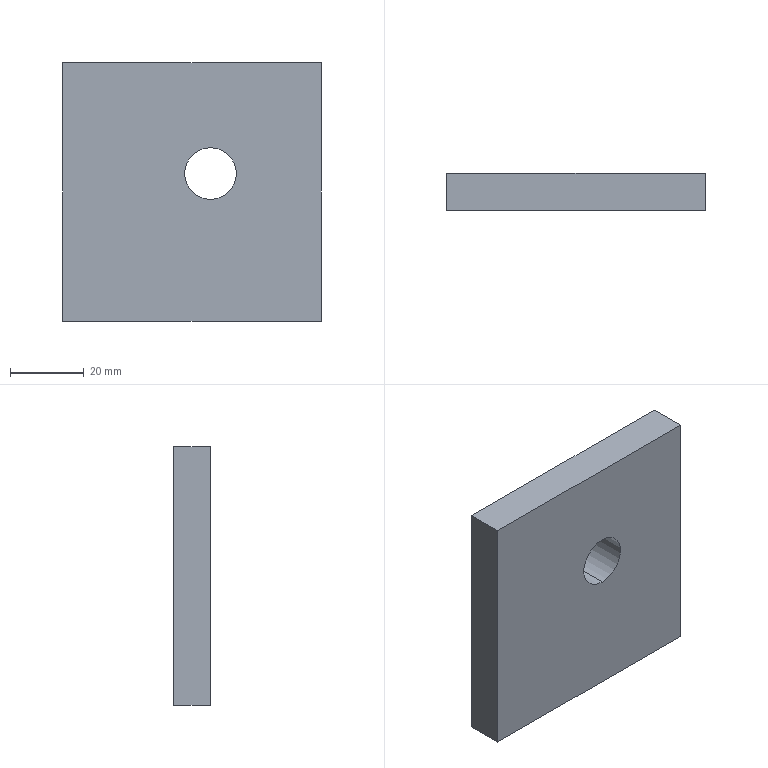Part | STEP file | PN_0078 foot-support plate | 1 solid | 8 faces | box 70 x 10 x 70 mm | volume 47461 mm3 | plane 6 | cylinder 2 | commonest cylinder face diameters 14 x2
STEP:
#1=CARTESIAN_POINT('',(0.,0.,0.));
#2=DIRECTION('',(0.,0.,1.));
#3=DIRECTION('',(1.,0.,0.));
#4=AXIS2_PLACEMENT_3D('',#1,#2,#3);
#5=CARTESIAN_POINT('',(-30.,0.,-23.));
#6=VERTEX_POINT('',#5);
#7=CARTESIAN_POINT('',(-30.,10.,-23.));
#8=VERTEX_POINT('',#7);
#9=CARTESIAN_POINT('',(-30.,10.,-23.));
#10=DIRECTION('',(0.,1.,0.));
#11=VECTOR('',#10,1.);
#12=LINE('',#9,#11);
#13=CARTESIAN_POINT('',(-30.,10.,-30.));
#14=DIRECTION('',(0.,1.,0.));
#15=DIRECTION('',(0.,0.,1.));
#16=AXIS2_PLACEMENT_3D('',#13,#14,#15);
#17=CYLINDRICAL_SURFACE('',#16,7.);
#18=CARTESIAN_POINT('',(6.283,0.));
#19=DIRECTION('',(0.,1.));
#20=VECTOR('',#19,1.);
#21=LINE('',#18,#20);
#22=(GEOMETRIC_REPRESENTATION_CONTEXT(2)PARAMETRIC_REPRESENTATION_CONTEXT()REPRESENTATION_CONTEXT('',''));
#23=DEFINITIONAL_REPRESENTATION('',(#21),#22);
#24=PCURVE('',#17,#23);
#25=CARTESIAN_POINT('',(-30.,10.,-30.));
#26=DIRECTION('',(0.,1.,0.));
#27=DIRECTION('',(0.,0.,1.));
#28=AXIS2_PLACEMENT_3D('',#25,#26,#27);
#29=CYLINDRICAL_SURFACE('',#28,7.);
#30=CARTESIAN_POINT('',(0.,0.));
#31=DIRECTION('',(0.,1.));
#32=VECTOR('',#31,1.);
#33=LINE('',#30,#32);
#34=(GEOMETRIC_REPRESENTATION_CONTEXT(2)PARAMETRIC_REPRESENTATION_CONTEXT()REPRESENTATION_CONTEXT('',''));
#35=DEFINITIONAL_REPRESENTATION('',(#33),#34);
#36=PCURVE('',#29,#35);
#37=SURFACE_CURVE('',#12,(#24,#36),.PCURVE_S1.);
#38=EDGE_CURVE('',#6,#8,#37,.T.);
#39=ORIENTED_EDGE('',*,*,#38,.T.);
#40=CARTESIAN_POINT('',(-30.,10.,-37.));
#41=VERTEX_POINT('',#40);
#42=CARTESIAN_POINT('',(-30.,10.,-30.));
#43=DIRECTION('',(0.,1.,0.));
#44=DIRECTION('',(0.,0.,1.));
#45=AXIS2_PLACEMENT_3D('',#42,#43,#44);
#46=CIRCLE('',#45,7.);
#47=CARTESIAN_POINT('',(0.,0.));
#48=DIRECTION('',(1.,0.));
#49=VECTOR('',#48,1.);
#50=LINE('',#47,#49);
#51=(GEOMETRIC_REPRESENTATION_CONTEXT(2)PARAMETRIC_REPRESENTATION_CONTEXT()REPRESENTATION_CONTEXT('',''));
#52=DEFINITIONAL_REPRESENTATION('',(#50),#51);
#53=PCURVE('',#17,#52);
#54=CARTESIAN_POINT('',(0.,10.,0.));
#55=DIRECTION('',(0.,1.,0.));
#56=DIRECTION('',(0.,0.,1.));
#57=AXIS2_PLACEMENT_3D('',#54,#55,#56);
#58=PLANE('',#57);
#59=CARTESIAN_POINT('',(-30.,-30.));
#60=DIRECTION('',(1.,0.));
#61=AXIS2_PLACEMENT_2D('',#59,#60);
#62=CIRCLE('',#61,7.);
#63=(GEOMETRIC_REPRESENTATION_CONTEXT(2)PARAMETRIC_REPRESENTATION_CONTEXT()REPRESENTATION_CONTEXT('',''));
#64=DEFINITIONAL_REPRESENTATION('',(#62),#63);
#65=PCURVE('',#58,#64);
#66=SURFACE_CURVE('',#46,(#53,#65),.PCURVE_S1.);
#67=EDGE_CURVE('',#41,#8,#66,.T.);
#68=ORIENTED_EDGE('',*,*,#67,.F.);
#69=CARTESIAN_POINT('',(-30.,0.,-37.));
#70=VERTEX_POINT('',#69);
#71=CARTESIAN_POINT('',(-30.,10.,-37.));
#72=DIRECTION('',(0.,1.,0.));
#73=VECTOR('',#72,1.);
#74=LINE('',#71,#73);
#75=CARTESIAN_POINT('',(3.142,0.));
#76=DIRECTION('',(0.,1.));
#77=VECTOR('',#76,1.);
#78=LINE('',#75,#77);
#79=(GEOMETRIC_REPRESENTATION_CONTEXT(2)PARAMETRIC_REPRESENTATION_CONTEXT()REPRESENTATION_CONTEXT('',''));
#80=DEFINITIONAL_REPRESENTATION('',(#78),#79);
#81=PCURVE('',#17,#80);
#82=CARTESIAN_POINT('',(3.142,0.));
#83=DIRECTION('',(0.,1.));
#84=VECTOR('',#83,1.);
#85=LINE('',#82,#84);
#86=(GEOMETRIC_REPRESENTATION_CONTEXT(2)PARAMETRIC_REPRESENTATION_CONTEXT()REPRESENTATION_CONTEXT('',''));
#87=DEFINITIONAL_REPRESENTATION('',(#85),#86);
#88=PCURVE('',#29,#87);
#89=SURFACE_CURVE('',#74,(#81,#88),.PCURVE_S1.);
#90=EDGE_CURVE('',#70,#41,#89,.T.);
#91=ORIENTED_EDGE('',*,*,#90,.F.);
#92=CARTESIAN_POINT('',(-30.,0.,-30.));
#93=DIRECTION('',(0.,1.,0.));
#94=DIRECTION('',(0.,0.,1.));
#95=AXIS2_PLACEMENT_3D('',#92,#93,#94);
#96=CIRCLE('',#95,7.);
#97=CARTESIAN_POINT('',(0.,-10.));
#98=DIRECTION('',(1.,0.));
#99=VECTOR('',#98,1.);
#100=LINE('',#97,#99);
#101=(GEOMETRIC_REPRESENTATION_CONTEXT(2)PARAMETRIC_REPRESENTATION_CONTEXT()REPRESENTATION_CONTEXT('',''));
#102=DEFINITIONAL_REPRESENTATION('',(#100),#101);
#103=PCURVE('',#17,#102);
#104=CARTESIAN_POINT('',(0.,0.,0.));
#105=DIRECTION('',(0.,1.,0.));
#106=DIRECTION('',(0.,0.,1.));
#107=AXIS2_PLACEMENT_3D('',#104,#105,#106);
#108=PLANE('',#107);
#109=CARTESIAN_POINT('',(-30.,-30.));
#110=DIRECTION('',(1.,0.));
#111=AXIS2_PLACEMENT_2D('',#109,#110);
#112=CIRCLE('',#111,7.);
#113=(GEOMETRIC_REPRESENTATION_CONTEXT(2)PARAMETRIC_REPRESENTATION_CONTEXT()REPRESENTATION_CONTEXT('',''));
#114=DEFINITIONAL_REPRESENTATION('',(#112),#113);
#115=PCURVE('',#108,#114);
#116=SURFACE_CURVE('',#96,(#103,#115),.PCURVE_S1.);
#117=EDGE_CURVE('',#70,#6,#116,.T.);
#118=ORIENTED_EDGE('',*,*,#117,.T.);
#119=EDGE_LOOP('',(#39,#68,#91,#118));
#120=FACE_BOUND('',#119,.F.);
#121=ADVANCED_FACE('',(#120),#17,.F.);
#122=CARTESIAN_POINT('',(0.,0.,0.));
#123=VERTEX_POINT('',#122);
#124=CARTESIAN_POINT('',(0.,0.,-70.));
#125=VERTEX_POINT('',#124);
#126=CARTESIAN_POINT('',(0.,0.,0.));
#127=DIRECTION('',(0.,0.,-1.));
#128=VECTOR('',#127,1.);
#129=LINE('',#126,#128);
#130=CARTESIAN_POINT('',(0.,10.,0.));
#131=DIRECTION('',(-1.,0.,0.));
#132=DIRECTION('',(0.,0.,1.));
#133=AXIS2_PLACEMENT_3D('',#130,#131,#132);
#134=PLANE('',#133);
#135=CARTESIAN_POINT('',(0.,-10.));
#136=DIRECTION('',(-1.,0.));
#137=VECTOR('',#136,1.);
#138=LINE('',#135,#137);
#139=(GEOMETRIC_REPRESENTATION_CONTEXT(2)PARAMETRIC_REPRESENTATION_CONTEXT()REPRESENTATION_CONTEXT('',''));
#140=DEFINITIONAL_REPRESENTATION('',(#138),#139);
#141=PCURVE('',#134,#140);
#142=CARTESIAN_POINT('',(0.,0.));
#143=DIRECTION('',(-1.,0.));
#144=VECTOR('',#143,1.);
#145=LINE('',#142,#144);
#146=(GEOMETRIC_REPRESENTATION_CONTEXT(2)PARAMETRIC_REPRESENTATION_CONTEXT()REPRESENTATION_CONTEXT('',''));
#147=DEFINITIONAL_REPRESENTATION('',(#145),#146);
#148=PCURVE('',#108,#147);
#149=SURFACE_CURVE('',#129,(#141,#148),.PCURVE_S1.);
#150=EDGE_CURVE('',#123,#125,#149,.T.);
#151=ORIENTED_EDGE('',*,*,#150,.T.);
#152=CARTESIAN_POINT('',(0.,10.,-70.));
#153=VERTEX_POINT('',#152);
#154=CARTESIAN_POINT('',(0.,10.,-70.));
#155=DIRECTION('',(0.,-1.,0.));
#156=VECTOR('',#155,1.);
#157=LINE('',#154,#156);
#158=CARTESIAN_POINT('',(-70.,0.));
#159=DIRECTION('',(0.,-1.));
#160=VECTOR('',#159,1.);
#161=LINE('',#158,#160);
#162=(GEOMETRIC_REPRESENTATION_CONTEXT(2)PARAMETRIC_REPRESENTATION_CONTEXT()REPRESENTATION_CONTEXT('',''));
#163=DEFINITIONAL_REPRESENTATION('',(#161),#162);
#164=PCURVE('',#134,#163);
#165=CARTESIAN_POINT('',(0.,10.,-70.));
#166=DIRECTION('',(0.,0.,1.));
#167=DIRECTION('',(1.,0.,0.));
#168=AXIS2_PLACEMENT_3D('',#165,#166,#167);
#169=PLANE('',#168);
#170=CARTESIAN_POINT('',(0.,0.));
#171=DIRECTION('',(0.,-1.));
#172=VECTOR('',#171,1.);
#173=LINE('',#170,#172);
#174=(GEOMETRIC_REPRESENTATION_CONTEXT(2)PARAMETRIC_REPRESENTATION_CONTEXT()REPRESENTATION_CONTEXT('',''));
#175=DEFINITIONAL_REPRESENTATION('',(#173),#174);
#176=PCURVE('',#169,#175);
#177=SURFACE_CURVE('',#157,(#164,#176),.PCURVE_S1.);
#178=EDGE_CURVE('',#153,#125,#177,.T.);
#179=ORIENTED_EDGE('',*,*,#178,.F.);
#180=CARTESIAN_POINT('',(0.,10.,0.));
#181=VERTEX_POINT('',#180);
#182=CARTESIAN_POINT('',(0.,10.,0.));
#183=DIRECTION('',(0.,0.,-1.));
#184=VECTOR('',#183,1.);
#185=LINE('',#182,#184);
#186=CARTESIAN_POINT('',(0.,0.));
#187=DIRECTION('',(-1.,0.));
#188=VECTOR('',#187,1.);
#189=LINE('',#186,#188);
#190=(GEOMETRIC_REPRESENTATION_CONTEXT(2)PARAMETRIC_REPRESENTATION_CONTEXT()REPRESENTATION_CONTEXT('',''));
#191=DEFINITIONAL_REPRESENTATION('',(#189),#190);
#192=PCURVE('',#134,#191);
#193=CARTESIAN_POINT('',(0.,0.));
#194=DIRECTION('',(-1.,0.));
#195=VECTOR('',#194,1.);
#196=LINE('',#193,#195);
#197=(GEOMETRIC_REPRESENTATION_CONTEXT(2)PARAMETRIC_REPRESENTATION_CONTEXT()REPRESENTATION_CONTEXT('',''));
#198=DEFINITIONAL_REPRESENTATION('',(#196),#197);
#199=PCURVE('',#58,#198);
#200=SURFACE_CURVE('',#185,(#192,#199),.PCURVE_S1.);
#201=EDGE_CURVE('',#181,#153,#200,.T.);
#202=ORIENTED_EDGE('',*,*,#201,.F.);
#203=CARTESIAN_POINT('',(0.,10.,0.));
#204=DIRECTION('',(0.,-1.,0.));
#205=VECTOR('',#204,1.);
#206=LINE('',#203,#205);
#207=CARTESIAN_POINT('',(0.,0.));
#208=DIRECTION('',(0.,-1.));
#209=VECTOR('',#208,1.);
#210=LINE('',#207,#209);
#211=(GEOMETRIC_REPRESENTATION_CONTEXT(2)PARAMETRIC_REPRESENTATION_CONTEXT()REPRESENTATION_CONTEXT('',''));
#212=DEFINITIONAL_REPRESENTATION('',(#210),#211);
#213=PCURVE('',#134,#212);
#214=CARTESIAN_POINT('',(0.,10.,0.));
#215=DIRECTION('',(0.,0.,-1.));
#216=DIRECTION('',(-1.,0.,0.));
#217=AXIS2_PLACEMENT_3D('',#214,#215,#216);
#218=PLANE('',#217);
#219=CARTESIAN_POINT('',(0.,0.));
#220=DIRECTION('',(0.,-1.));
#221=VECTOR('',#220,1.);
#222=LINE('',#219,#221);
#223=(GEOMETRIC_REPRESENTATION_CONTEXT(2)PARAMETRIC_REPRESENTATION_CONTEXT()REPRESENTATION_CONTEXT('',''));
#224=DEFINITIONAL_REPRESENTATION('',(#222),#223);
#225=PCURVE('',#218,#224);
#226=SURFACE_CURVE('',#206,(#213,#225),.PCURVE_S1.);
#227=EDGE_CURVE('',#181,#123,#226,.T.);
#228=ORIENTED_EDGE('',*,*,#227,.T.);
#229=EDGE_LOOP('',(#151,#179,#202,#228));
#230=FACE_BOUND('',#229,.T.);
#231=ADVANCED_FACE('',(#230),#134,.F.);
#232=CARTESIAN_POINT('',(-70.,0.,-70.));
#233=VERTEX_POINT('',#232);
#234=CARTESIAN_POINT('',(0.,0.,-70.));
#235=DIRECTION('',(-1.,0.,0.));
#236=VECTOR('',#235,1.);
#237=LINE('',#234,#236);
#238=CARTESIAN_POINT('',(0.,-10.));
#239=DIRECTION('',(-1.,0.));
#240=VECTOR('',#239,1.);
#241=LINE('',#238,#240);
#242=(GEOMETRIC_REPRESENTATION_CONTEXT(2)PARAMETRIC_REPRESENTATION_CONTEXT()REPRESENTATION_CONTEXT('',''));
#243=DEFINITIONAL_REPRESENTATION('',(#241),#242);
#244=PCURVE('',#169,#243);
#245=CARTESIAN_POINT('',(-70.,0.));
#246=DIRECTION('',(0.,-1.));
#247=VECTOR('',#246,1.);
#248=LINE('',#245,#247);
#249=(GEOMETRIC_REPRESENTATION_CONTEXT(2)PARAMETRIC_REPRESENTATION_CONTEXT()REPRESENTATION_CONTEXT('',''));
#250=DEFINITIONAL_REPRESENTATION('',(#248),#249);
#251=PCURVE('',#108,#250);
#252=SURFACE_CURVE('',#237,(#244,#251),.PCURVE_S1.);
#253=EDGE_CURVE('',#125,#233,#252,.T.);
#254=ORIENTED_EDGE('',*,*,#253,.T.);
#255=CARTESIAN_POINT('',(-70.,10.,-70.));
#256=VERTEX_POINT('',#255);
#257=CARTESIAN_POINT('',(-70.,10.,-70.));
#258=DIRECTION('',(0.,-1.,0.));
#259=VECTOR('',#258,1.);
#260=LINE('',#257,#259);
#261=CARTESIAN_POINT('',(-70.,0.));
#262=DIRECTION('',(0.,-1.));
#263=VECTOR('',#262,1.);
#264=LINE('',#261,#263);
#265=(GEOMETRIC_REPRESENTATION_CONTEXT(2)PARAMETRIC_REPRESENTATION_CONTEXT()REPRESENTATION_CONTEXT('',''));
#266=DEFINITIONAL_REPRESENTATION('',(#264),#265);
#267=PCURVE('',#169,#266);
#268=CARTESIAN_POINT('',(-70.,10.,0.));
#269=DIRECTION('',(1.,0.,0.));
#270=DIRECTION('',(0.,0.,-1.));
#271=AXIS2_PLACEMENT_3D('',#268,#269,#270);
#272=PLANE('',#271);
#273=CARTESIAN_POINT('',(70.,0.));
#274=DIRECTION('',(0.,-1.));
#275=VECTOR('',#274,1.);
#276=LINE('',#273,#275);
#277=(GEOMETRIC_REPRESENTATION_CONTEXT(2)PARAMETRIC_REPRESENTATION_CONTEXT()REPRESENTATION_CONTEXT('',''));
#278=DEFINITIONAL_REPRESENTATION('',(#276),#277);
#279=PCURVE('',#272,#278);
#280=SURFACE_CURVE('',#260,(#267,#279),.PCURVE_S1.);
#281=EDGE_CURVE('',#256,#233,#280,.T.);
#282=ORIENTED_EDGE('',*,*,#281,.F.);
#283=CARTESIAN_POINT('',(0.,10.,-70.));
#284=DIRECTION('',(-1.,0.,0.));
#285=VECTOR('',#284,1.);
#286=LINE('',#283,#285);
#287=CARTESIAN_POINT('',(0.,0.));
#288=DIRECTION('',(-1.,0.));
#289=VECTOR('',#288,1.);
#290=LINE('',#287,#289);
#291=(GEOMETRIC_REPRESENTATION_CONTEXT(2)PARAMETRIC_REPRESENTATION_CONTEXT()REPRESENTATION_CONTEXT('',''));
#292=DEFINITIONAL_REPRESENTATION('',(#290),#291);
#293=PCURVE('',#169,#292);
#294=CARTESIAN_POINT('',(-70.,0.));
#295=DIRECTION('',(0.,-1.));
#296=VECTOR('',#295,1.);
#297=LINE('',#294,#296);
#298=(GEOMETRIC_REPRESENTATION_CONTEXT(2)PARAMETRIC_REPRESENTATION_CONTEXT()REPRESENTATION_CONTEXT('',''));
#299=DEFINITIONAL_REPRESENTATION('',(#297),#298);
#300=PCURVE('',#58,#299);
#301=SURFACE_CURVE('',#286,(#293,#300),.PCURVE_S1.);
#302=EDGE_CURVE('',#153,#256,#301,.T.);
#303=ORIENTED_EDGE('',*,*,#302,.F.);
#304=ORIENTED_EDGE('',*,*,#178,.T.);
#305=EDGE_LOOP('',(#254,#282,#303,#304));
#306=FACE_BOUND('',#305,.T.);
#307=ADVANCED_FACE('',(#306),#169,.F.);
#308=CARTESIAN_POINT('',(-70.,0.,0.));
#309=VERTEX_POINT('',#308);
#310=CARTESIAN_POINT('',(-70.,0.,0.));
#311=DIRECTION('',(0.,0.,1.));
#312=VECTOR('',#311,1.);
#313=LINE('',#310,#312);
#314=CARTESIAN_POINT('',(0.,-10.));
#315=DIRECTION('',(-1.,0.));
#316=VECTOR('',#315,1.);
#317=LINE('',#314,#316);
#318=(GEOMETRIC_REPRESENTATION_CONTEXT(2)PARAMETRIC_REPRESENTATION_CONTEXT()REPRESENTATION_CONTEXT('',''));
#319=DEFINITIONAL_REPRESENTATION('',(#317),#318);
#320=PCURVE('',#272,#319);
#321=CARTESIAN_POINT('',(0.,-70.));
#322=DIRECTION('',(1.,0.));
#323=VECTOR('',#322,1.);
#324=LINE('',#321,#323);
#325=(GEOMETRIC_REPRESENTATION_CONTEXT(2)PARAMETRIC_REPRESENTATION_CONTEXT()REPRESENTATION_CONTEXT('',''));
#326=DEFINITIONAL_REPRESENTATION('',(#324),#325);
#327=PCURVE('',#108,#326);
#328=SURFACE_CURVE('',#313,(#320,#327),.PCURVE_S1.);
#329=EDGE_CURVE('',#233,#309,#328,.T.);
#330=ORIENTED_EDGE('',*,*,#329,.T.);
#331=CARTESIAN_POINT('',(-70.,10.,0.));
#332=VERTEX_POINT('',#331);
#333=CARTESIAN_POINT('',(-70.,10.,0.));
#334=DIRECTION('',(0.,-1.,0.));
#335=VECTOR('',#334,1.);
#336=LINE('',#333,#335);
#337=CARTESIAN_POINT('',(0.,0.));
#338=DIRECTION('',(0.,-1.));
#339=VECTOR('',#338,1.);
#340=LINE('',#337,#339);
#341=(GEOMETRIC_REPRESENTATION_CONTEXT(2)PARAMETRIC_REPRESENTATION_CONTEXT()REPRESENTATION_CONTEXT('',''));
#342=DEFINITIONAL_REPRESENTATION('',(#340),#341);
#343=PCURVE('',#272,#342);
#344=CARTESIAN_POINT('',(70.,0.));
#345=DIRECTION('',(0.,-1.));
#346=VECTOR('',#345,1.);
#347=LINE('',#344,#346);
#348=(GEOMETRIC_REPRESENTATION_CONTEXT(2)PARAMETRIC_REPRESENTATION_CONTEXT()REPRESENTATION_CONTEXT('',''));
#349=DEFINITIONAL_REPRESENTATION('',(#347),#348);
#350=PCURVE('',#218,#349);
#351=SURFACE_CURVE('',#336,(#343,#350),.PCURVE_S1.);
#352=EDGE_CURVE('',#332,#309,#351,.T.);
#353=ORIENTED_EDGE('',*,*,#352,.F.);
#354=CARTESIAN_POINT('',(-70.,10.,0.));
#355=DIRECTION('',(0.,0.,1.));
#356=VECTOR('',#355,1.);
#357=LINE('',#354,#356);
#358=CARTESIAN_POINT('',(0.,0.));
#359=DIRECTION('',(-1.,0.));
#360=VECTOR('',#359,1.);
#361=LINE('',#358,#360);
#362=(GEOMETRIC_REPRESENTATION_CONTEXT(2)PARAMETRIC_REPRESENTATION_CONTEXT()REPRESENTATION_CONTEXT('',''));
#363=DEFINITIONAL_REPRESENTATION('',(#361),#362);
#364=PCURVE('',#272,#363);
#365=CARTESIAN_POINT('',(0.,-70.));
#366=DIRECTION('',(1.,0.));
#367=VECTOR('',#366,1.);
#368=LINE('',#365,#367);
#369=(GEOMETRIC_REPRESENTATION_CONTEXT(2)PARAMETRIC_REPRESENTATION_CONTEXT()REPRESENTATION_CONTEXT('',''));
#370=DEFINITIONAL_REPRESENTATION('',(#368),#369);
#371=PCURVE('',#58,#370);
#372=SURFACE_CURVE('',#357,(#364,#371),.PCURVE_S1.);
#373=EDGE_CURVE('',#256,#332,#372,.T.);
#374=ORIENTED_EDGE('',*,*,#373,.F.);
#375=ORIENTED_EDGE('',*,*,#281,.T.);
#376=EDGE_LOOP('',(#330,#353,#374,#375));
#377=FACE_BOUND('',#376,.T.);
#378=ADVANCED_FACE('',(#377),#272,.F.);
#379=CARTESIAN_POINT('',(0.,0.,0.));
#380=DIRECTION('',(1.,0.,0.));
#381=VECTOR('',#380,1.);
#382=LINE('',#379,#381);
#383=CARTESIAN_POINT('',(0.,-10.));
#384=DIRECTION('',(-1.,0.));
#385=VECTOR('',#384,1.);
#386=LINE('',#383,#385);
#387=(GEOMETRIC_REPRESENTATION_CONTEXT(2)PARAMETRIC_REPRESENTATION_CONTEXT()REPRESENTATION_CONTEXT('',''));
#388=DEFINITIONAL_REPRESENTATION('',(#386),#387);
#389=PCURVE('',#218,#388);
#390=CARTESIAN_POINT('',(0.,0.));
#391=DIRECTION('',(0.,1.));
#392=VECTOR('',#391,1.);
#393=LINE('',#390,#392);
#394=(GEOMETRIC_REPRESENTATION_CONTEXT(2)PARAMETRIC_REPRESENTATION_CONTEXT()REPRESENTATION_CONTEXT('',''));
#395=DEFINITIONAL_REPRESENTATION('',(#393),#394);
#396=PCURVE('',#108,#395);
#397=SURFACE_CURVE('',#382,(#389,#396),.PCURVE_S1.);
#398=EDGE_CURVE('',#309,#123,#397,.T.);
#399=ORIENTED_EDGE('',*,*,#398,.T.);
#400=ORIENTED_EDGE('',*,*,#227,.F.);
#401=CARTESIAN_POINT('',(0.,10.,0.));
#402=DIRECTION('',(1.,0.,0.));
#403=VECTOR('',#402,1.);
#404=LINE('',#401,#403);
#405=CARTESIAN_POINT('',(0.,0.));
#406=DIRECTION('',(-1.,0.));
#407=VECTOR('',#406,1.);
#408=LINE('',#405,#407);
#409=(GEOMETRIC_REPRESENTATION_CONTEXT(2)PARAMETRIC_REPRESENTATION_CONTEXT()REPRESENTATION_CONTEXT('',''));
#410=DEFINITIONAL_REPRESENTATION('',(#408),#409);
#411=PCURVE('',#218,#410);
#412=CARTESIAN_POINT('',(0.,0.));
#413=DIRECTION('',(0.,1.));
#414=VECTOR('',#413,1.);
#415=LINE('',#412,#414);
#416=(GEOMETRIC_REPRESENTATION_CONTEXT(2)PARAMETRIC_REPRESENTATION_CONTEXT()REPRESENTATION_CONTEXT('',''));
#417=DEFINITIONAL_REPRESENTATION('',(#415),#416);
#418=PCURVE('',#58,#417);
#419=SURFACE_CURVE('',#404,(#411,#418),.PCURVE_S1.);
#420=EDGE_CURVE('',#332,#181,#419,.T.);
#421=ORIENTED_EDGE('',*,*,#420,.F.);
#422=ORIENTED_EDGE('',*,*,#352,.T.);
#423=EDGE_LOOP('',(#399,#400,#421,#422));
#424=FACE_BOUND('',#423,.T.);
#425=ADVANCED_FACE('',(#424),#218,.F.);
#426=CARTESIAN_POINT('',(-30.,10.,-30.));
#427=DIRECTION('',(0.,1.,0.));
#428=DIRECTION('',(0.,0.,1.));
#429=AXIS2_PLACEMENT_3D('',#426,#427,#428);
#430=CIRCLE('',#429,7.);
#431=CARTESIAN_POINT('',(-30.,-30.));
#432=DIRECTION('',(1.,0.));
#433=AXIS2_PLACEMENT_2D('',#431,#432);
#434=CIRCLE('',#433,7.);
#435=(GEOMETRIC_REPRESENTATION_CONTEXT(2)PARAMETRIC_REPRESENTATION_CONTEXT()REPRESENTATION_CONTEXT('',''));
#436=DEFINITIONAL_REPRESENTATION('',(#434),#435);
#437=PCURVE('',#58,#436);
#438=CARTESIAN_POINT('',(0.,0.));
#439=DIRECTION('',(1.,0.));
#440=VECTOR('',#439,1.);
#441=LINE('',#438,#440);
#442=(GEOMETRIC_REPRESENTATION_CONTEXT(2)PARAMETRIC_REPRESENTATION_CONTEXT()REPRESENTATION_CONTEXT('',''));
#443=DEFINITIONAL_REPRESENTATION('',(#441),#442);
#444=PCURVE('',#29,#443);
#445=SURFACE_CURVE('',#430,(#437,#444),.PCURVE_S1.);
#446=EDGE_CURVE('',#8,#41,#445,.T.);
#447=ORIENTED_EDGE('',*,*,#446,.F.);
#448=ORIENTED_EDGE('',*,*,#67,.F.);
#449=EDGE_LOOP('',(#447,#448));
#450=FACE_BOUND('',#449,.T.);
#451=ORIENTED_EDGE('',*,*,#201,.T.);
#452=ORIENTED_EDGE('',*,*,#302,.T.);
#453=ORIENTED_EDGE('',*,*,#373,.T.);
#454=ORIENTED_EDGE('',*,*,#420,.T.);
#455=EDGE_LOOP('',(#451,#452,#453,#454));
#456=FACE_BOUND('',#455,.T.);
#457=ADVANCED_FACE('',(#450,#456),#58,.T.);
#458=CARTESIAN_POINT('',(-30.,0.,-30.));
#459=DIRECTION('',(0.,1.,0.));
#460=DIRECTION('',(0.,0.,1.));
#461=AXIS2_PLACEMENT_3D('',#458,#459,#460);
#462=CIRCLE('',#461,7.);
#463=CARTESIAN_POINT('',(-30.,-30.));
#464=DIRECTION('',(1.,0.));
#465=AXIS2_PLACEMENT_2D('',#463,#464);
#466=CIRCLE('',#465,7.);
#467=(GEOMETRIC_REPRESENTATION_CONTEXT(2)PARAMETRIC_REPRESENTATION_CONTEXT()REPRESENTATION_CONTEXT('',''));
#468=DEFINITIONAL_REPRESENTATION('',(#466),#467);
#469=PCURVE('',#108,#468);
#470=CARTESIAN_POINT('',(0.,-10.));
#471=DIRECTION('',(1.,0.));
#472=VECTOR('',#471,1.);
#473=LINE('',#470,#472);
#474=(GEOMETRIC_REPRESENTATION_CONTEXT(2)PARAMETRIC_REPRESENTATION_CONTEXT()REPRESENTATION_CONTEXT('',''));
#475=DEFINITIONAL_REPRESENTATION('',(#473),#474);
#476=PCURVE('',#29,#475);
#477=SURFACE_CURVE('',#462,(#469,#476),.PCURVE_S1.);
#478=EDGE_CURVE('',#6,#70,#477,.T.);
#479=ORIENTED_EDGE('',*,*,#478,.T.);
#480=ORIENTED_EDGE('',*,*,#117,.T.);
#481=EDGE_LOOP('',(#479,#480));
#482=FACE_BOUND('',#481,.T.);
#483=ORIENTED_EDGE('',*,*,#150,.F.);
#484=ORIENTED_EDGE('',*,*,#398,.F.);
#485=ORIENTED_EDGE('',*,*,#329,.F.);
#486=ORIENTED_EDGE('',*,*,#253,.F.);
#487=EDGE_LOOP('',(#483,#484,#485,#486));
#488=FACE_BOUND('',#487,.T.);
#489=ADVANCED_FACE('',(#482,#488),#108,.F.);
#490=ORIENTED_EDGE('',*,*,#446,.F.);
#491=ORIENTED_EDGE('',*,*,#38,.F.);
#492=ORIENTED_EDGE('',*,*,#478,.T.);
#493=ORIENTED_EDGE('',*,*,#90,.T.);
#494=EDGE_LOOP('',(#490,#491,#492,#493));
#495=FACE_BOUND('',#494,.F.);
#496=ADVANCED_FACE('',(#495),#29,.F.);
#497=CLOSED_SHELL('',(#121,#231,#307,#378,#425,#457,#489,#496));
#498=MANIFOLD_SOLID_BREP('',#497);
#499=(LENGTH_UNIT()NAMED_UNIT(*)SI_UNIT(.MILLI.,.METRE.));
#500=UNCERTAINTY_MEASURE_WITH_UNIT(LENGTH_MEASURE(0.0000001),#499,'','');
#501=(NAMED_UNIT(*)PLANE_ANGLE_UNIT()SI_UNIT($,.RADIAN.));
#502=(NAMED_UNIT(*)SI_UNIT($,.STERADIAN.)SOLID_ANGLE_UNIT());
#503=(GEOMETRIC_REPRESENTATION_CONTEXT(3)GLOBAL_UNCERTAINTY_ASSIGNED_CONTEXT((#500))GLOBAL_UNIT_ASSIGNED_CONTEXT((#499,#501,#502))REPRESENTATION_CONTEXT('',''));
#504=ADVANCED_BREP_SHAPE_REPRESENTATION('',(#4,#498),#503);